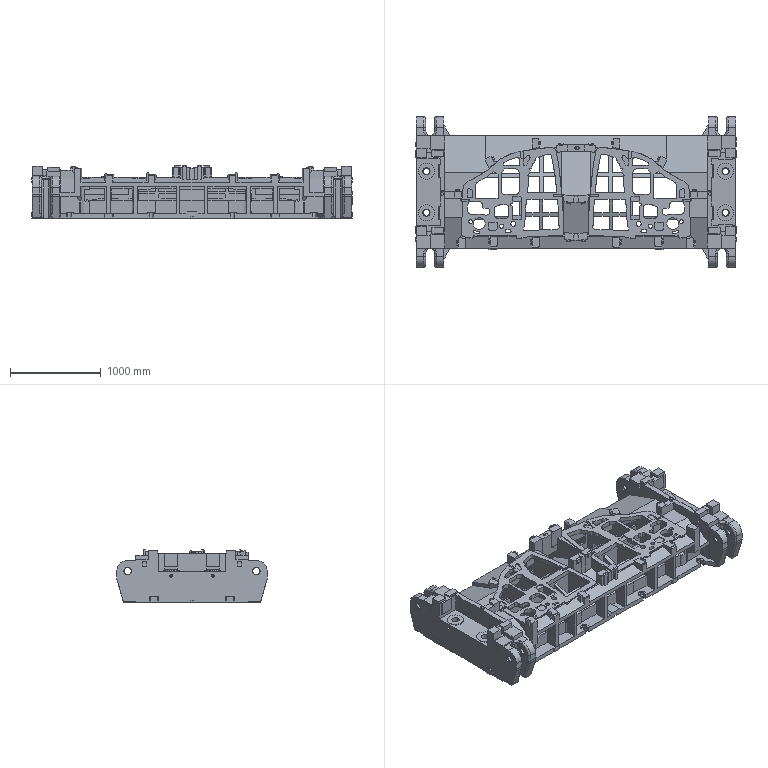Part | NX | features solid 2 | 1 solid | 2048 faces | box 3540 x 1660 x 575 mm | volume 762145509 mm3 | plane 1465 | cylinder 417 | spline 138 | torus 28 | commonest cylinder face diameters 40 x158 83 x48 80 x42 60 x38 100 x32 79 x16